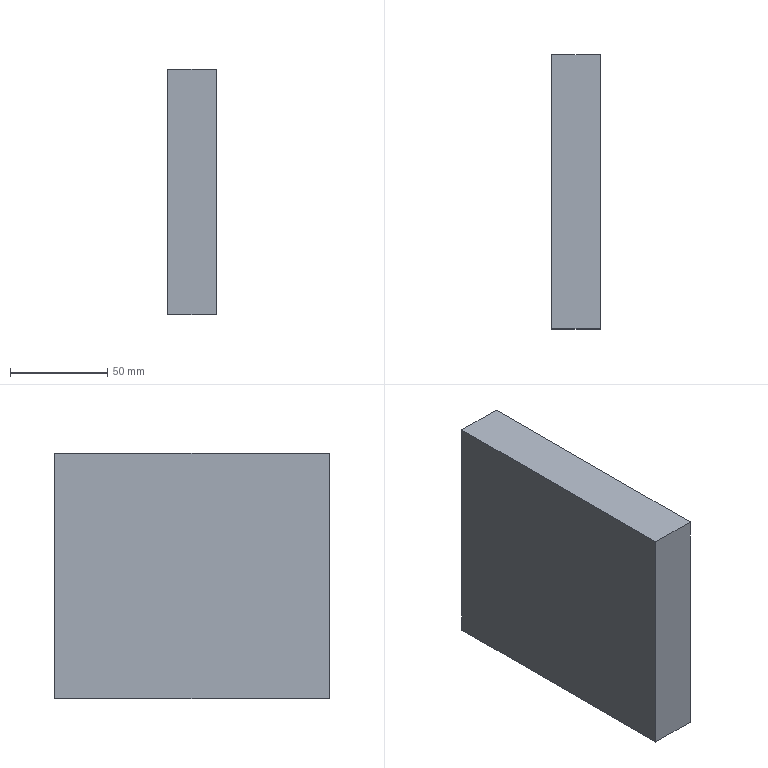Part | SolidWorks | features Extrusion 1 | 1 solid | 6 faces | box 25 x 141 x 126 mm | volume 444150 mm3 | plane 6
STEP:
#1=CARTESIAN_POINT('',(-12.5,-70.5,-63.));
#2=VERTEX_POINT('',#1);
#3=CARTESIAN_POINT('',(-12.5,-70.5,63.));
#4=VERTEX_POINT('',#3);
#5=CARTESIAN_POINT('',(-12.5,-70.5,-63.));
#6=DIRECTION('',(0.,0.,1.));
#7=VECTOR('',#6,1000.);
#8=LINE('',#5,#7);
#9=EDGE_CURVE('',#2,#4,#8,.T.);
#10=ORIENTED_EDGE('',*,*,#9,.T.);
#11=CARTESIAN_POINT('',(-12.5,70.5,63.));
#12=VERTEX_POINT('',#11);
#13=CARTESIAN_POINT('',(-12.5,70.5,63.));
#14=DIRECTION('',(0.,-1.,0.));
#15=VECTOR('',#14,1000.);
#16=LINE('',#13,#15);
#17=EDGE_CURVE('',#12,#4,#16,.T.);
#18=ORIENTED_EDGE('',*,*,#17,.F.);
#19=CARTESIAN_POINT('',(-12.5,70.5,-63.));
#20=VERTEX_POINT('',#19);
#21=CARTESIAN_POINT('',(-12.5,70.5,-63.));
#22=DIRECTION('',(0.,0.,1.));
#23=VECTOR('',#22,1000.);
#24=LINE('',#21,#23);
#25=EDGE_CURVE('',#20,#12,#24,.T.);
#26=ORIENTED_EDGE('',*,*,#25,.F.);
#27=CARTESIAN_POINT('',(-12.5,70.5,-63.));
#28=DIRECTION('',(0.,-1.,0.));
#29=VECTOR('',#28,1000.);
#30=LINE('',#27,#29);
#31=EDGE_CURVE('',#20,#2,#30,.T.);
#32=ORIENTED_EDGE('',*,*,#31,.T.);
#33=EDGE_LOOP('',(#10,#18,#26,#32));
#34=FACE_OUTER_BOUND('',#33,.T.);
#35=CARTESIAN_POINT('',(-12.5,70.5,-63.));
#36=DIRECTION('',(1.,0.,0.));
#37=DIRECTION('',(0.,0.,-1.));
#38=AXIS2_PLACEMENT_3D('',#35,#36,#37);
#39=PLANE('',#38);
#40=ADVANCED_FACE('',(#34),#39,.F.);
#41=CARTESIAN_POINT('',(12.5,-70.5,63.));
#42=VERTEX_POINT('',#41);
#43=CARTESIAN_POINT('',(-12.5,-70.5,63.));
#44=DIRECTION('',(1.,0.,0.));
#45=VECTOR('',#44,1000.);
#46=LINE('',#43,#45);
#47=EDGE_CURVE('',#4,#42,#46,.T.);
#48=ORIENTED_EDGE('',*,*,#47,.T.);
#49=CARTESIAN_POINT('',(12.5,70.5,63.));
#50=VERTEX_POINT('',#49);
#51=CARTESIAN_POINT('',(12.5,70.5,63.));
#52=DIRECTION('',(0.,-1.,0.));
#53=VECTOR('',#52,1000.);
#54=LINE('',#51,#53);
#55=EDGE_CURVE('',#50,#42,#54,.T.);
#56=ORIENTED_EDGE('',*,*,#55,.F.);
#57=CARTESIAN_POINT('',(-12.5,70.5,63.));
#58=DIRECTION('',(1.,0.,0.));
#59=VECTOR('',#58,1000.);
#60=LINE('',#57,#59);
#61=EDGE_CURVE('',#12,#50,#60,.T.);
#62=ORIENTED_EDGE('',*,*,#61,.F.);
#63=ORIENTED_EDGE('',*,*,#17,.T.);
#64=EDGE_LOOP('',(#48,#56,#62,#63));
#65=FACE_OUTER_BOUND('',#64,.T.);
#66=CARTESIAN_POINT('',(-12.5,70.5,63.));
#67=DIRECTION('',(0.,0.,-1.));
#68=DIRECTION('',(-1.,0.,0.));
#69=AXIS2_PLACEMENT_3D('',#66,#67,#68);
#70=PLANE('',#69);
#71=ADVANCED_FACE('',(#65),#70,.F.);
#72=CARTESIAN_POINT('',(12.5,-70.5,-63.));
#73=VERTEX_POINT('',#72);
#74=CARTESIAN_POINT('',(12.5,-70.5,-63.));
#75=DIRECTION('',(0.,0.,-1.));
#76=VECTOR('',#75,1000.);
#77=LINE('',#74,#76);
#78=EDGE_CURVE('',#42,#73,#77,.T.);
#79=ORIENTED_EDGE('',*,*,#78,.T.);
#80=CARTESIAN_POINT('',(12.5,70.5,-63.));
#81=VERTEX_POINT('',#80);
#82=CARTESIAN_POINT('',(12.5,70.5,-63.));
#83=DIRECTION('',(0.,-1.,0.));
#84=VECTOR('',#83,1000.);
#85=LINE('',#82,#84);
#86=EDGE_CURVE('',#81,#73,#85,.T.);
#87=ORIENTED_EDGE('',*,*,#86,.F.);
#88=CARTESIAN_POINT('',(12.5,70.5,-63.));
#89=DIRECTION('',(0.,0.,-1.));
#90=VECTOR('',#89,1000.);
#91=LINE('',#88,#90);
#92=EDGE_CURVE('',#50,#81,#91,.T.);
#93=ORIENTED_EDGE('',*,*,#92,.F.);
#94=ORIENTED_EDGE('',*,*,#55,.T.);
#95=EDGE_LOOP('',(#79,#87,#93,#94));
#96=FACE_OUTER_BOUND('',#95,.T.);
#97=CARTESIAN_POINT('',(12.5,70.5,-63.));
#98=DIRECTION('',(-1.,0.,0.));
#99=DIRECTION('',(0.,0.,1.));
#100=AXIS2_PLACEMENT_3D('',#97,#98,#99);
#101=PLANE('',#100);
#102=ADVANCED_FACE('',(#96),#101,.F.);
#103=CARTESIAN_POINT('',(-12.5,-70.5,-63.));
#104=DIRECTION('',(-1.,0.,0.));
#105=VECTOR('',#104,1000.);
#106=LINE('',#103,#105);
#107=EDGE_CURVE('',#73,#2,#106,.T.);
#108=ORIENTED_EDGE('',*,*,#107,.T.);
#109=ORIENTED_EDGE('',*,*,#31,.F.);
#110=CARTESIAN_POINT('',(-12.5,70.5,-63.));
#111=DIRECTION('',(-1.,0.,0.));
#112=VECTOR('',#111,1000.);
#113=LINE('',#110,#112);
#114=EDGE_CURVE('',#81,#20,#113,.T.);
#115=ORIENTED_EDGE('',*,*,#114,.F.);
#116=ORIENTED_EDGE('',*,*,#86,.T.);
#117=EDGE_LOOP('',(#108,#109,#115,#116));
#118=FACE_OUTER_BOUND('',#117,.T.);
#119=CARTESIAN_POINT('',(-12.5,70.5,-63.));
#120=DIRECTION('',(0.,0.,1.));
#121=DIRECTION('',(1.,0.,0.));
#122=AXIS2_PLACEMENT_3D('',#119,#120,#121);
#123=PLANE('',#122);
#124=ADVANCED_FACE('',(#118),#123,.F.);
#125=ORIENTED_EDGE('',*,*,#25,.T.);
#126=ORIENTED_EDGE('',*,*,#61,.T.);
#127=ORIENTED_EDGE('',*,*,#92,.T.);
#128=ORIENTED_EDGE('',*,*,#114,.T.);
#129=EDGE_LOOP('',(#125,#126,#127,#128));
#130=FACE_OUTER_BOUND('',#129,.T.);
#131=CARTESIAN_POINT('',(0.,70.5,0.));
#132=DIRECTION('',(0.,1.,0.));
#133=DIRECTION('',(0.,0.,1.));
#134=AXIS2_PLACEMENT_3D('',#131,#132,#133);
#135=PLANE('',#134);
#136=ADVANCED_FACE('',(#130),#135,.T.);
#137=ORIENTED_EDGE('',*,*,#9,.F.);
#138=ORIENTED_EDGE('',*,*,#107,.F.);
#139=ORIENTED_EDGE('',*,*,#78,.F.);
#140=ORIENTED_EDGE('',*,*,#47,.F.);
#141=EDGE_LOOP('',(#137,#138,#139,#140));
#142=FACE_OUTER_BOUND('',#141,.T.);
#143=CARTESIAN_POINT('',(0.,-70.5,0.));
#144=DIRECTION('',(0.,1.,0.));
#145=DIRECTION('',(0.,0.,1.));
#146=AXIS2_PLACEMENT_3D('',#143,#144,#145);
#147=PLANE('',#146);
#148=ADVANCED_FACE('',(#142),#147,.F.);
#149=CLOSED_SHELL('',(#40,#71,#102,#124,#136,#148));
#150=MANIFOLD_SOLID_BREP('',#149);
#151=CARTESIAN_POINT('',(0.,0.,0.));
#152=DIRECTION('',(0.,0.,1.));
#153=DIRECTION('',(1.,0.,0.));
#154=AXIS2_PLACEMENT_3D('',#151,#152,#153);
#155=(LENGTH_UNIT()NAMED_UNIT(*)SI_UNIT(.MILLI.,.METRE.));
#156=UNCERTAINTY_MEASURE_WITH_UNIT(LENGTH_MEASURE(0.00001),#155,'','');
#157=(NAMED_UNIT(*)PLANE_ANGLE_UNIT()SI_UNIT($,.RADIAN.));
#158=(NAMED_UNIT(*)SI_UNIT($,.STERADIAN.)SOLID_ANGLE_UNIT());
#159=(GEOMETRIC_REPRESENTATION_CONTEXT(3)GLOBAL_UNCERTAINTY_ASSIGNED_CONTEXT((#156))GLOBAL_UNIT_ASSIGNED_CONTEXT((#155,#157,#158))REPRESENTATION_CONTEXT('',''));
#160=ADVANCED_BREP_SHAPE_REPRESENTATION('',(#150,#154),#159);